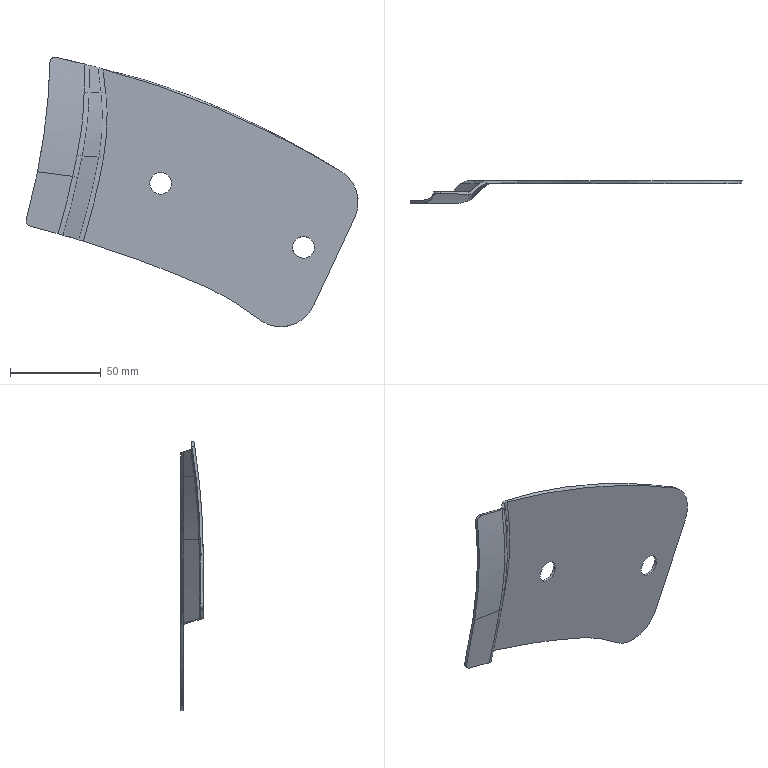Part | STEP file | FNA5401871 | 1 solid | 53 faces | box 183.449 x 12.361 x 148.782 mm | volume 24633 mm3 | spline 37 | cylinder 6 | other 6 | plane 4 | commonest cylinder face diameters 12 x4 8 x1 11 x1